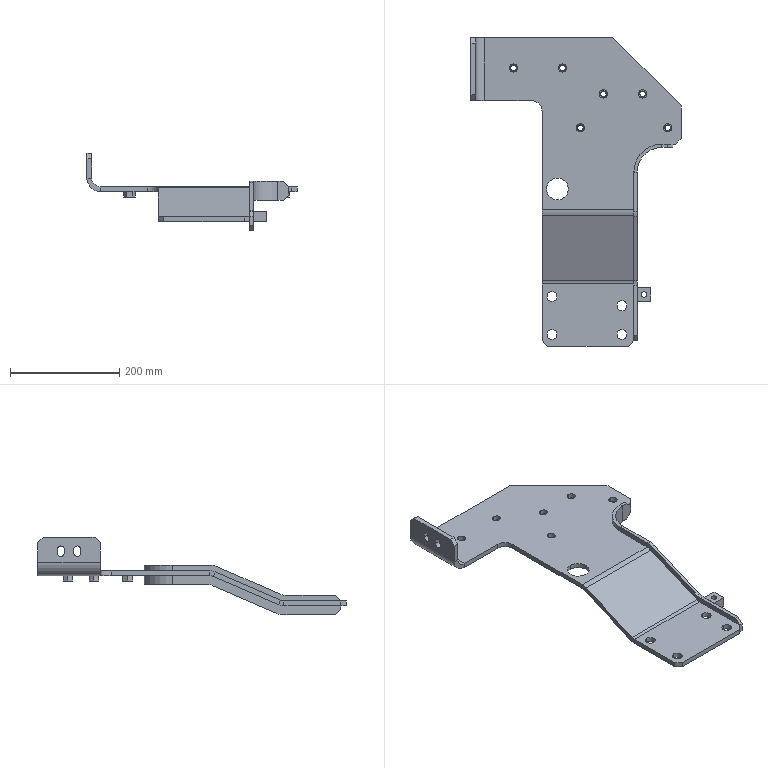Part | SolidWorks | features BaseBody 9, CosmeticWeldCutList 1 | 9 solids | 516 faces | box 385 x 565 x 141 mm | volume 1220109 mm3 | cone 264 | cylinder 140 | plane 112 | commonest cylinder face diameters 10.106 x96 15 x12 18 x8 50 x7 12.5 x6 32 x3